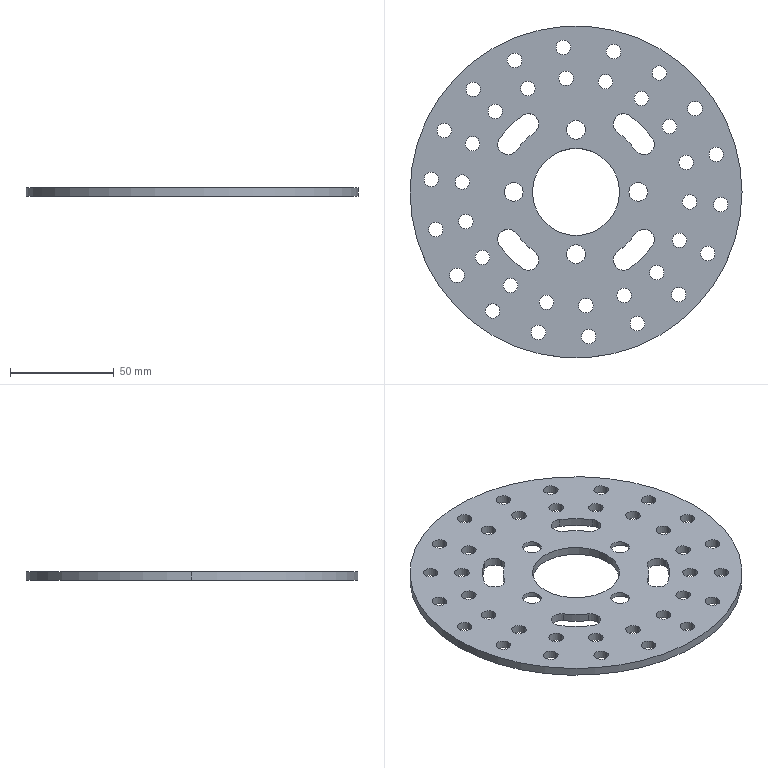Part | SolidWorks | features BaseBody 1 | 1 solid | 118 faces | box 160 x 160 x 4 mm | volume 64110 mm3 | cylinder 112 | plane 6 | commonest cylinder face diameters 7 x72 10 x12 9 x8 14 x8 70 x4 90 x4